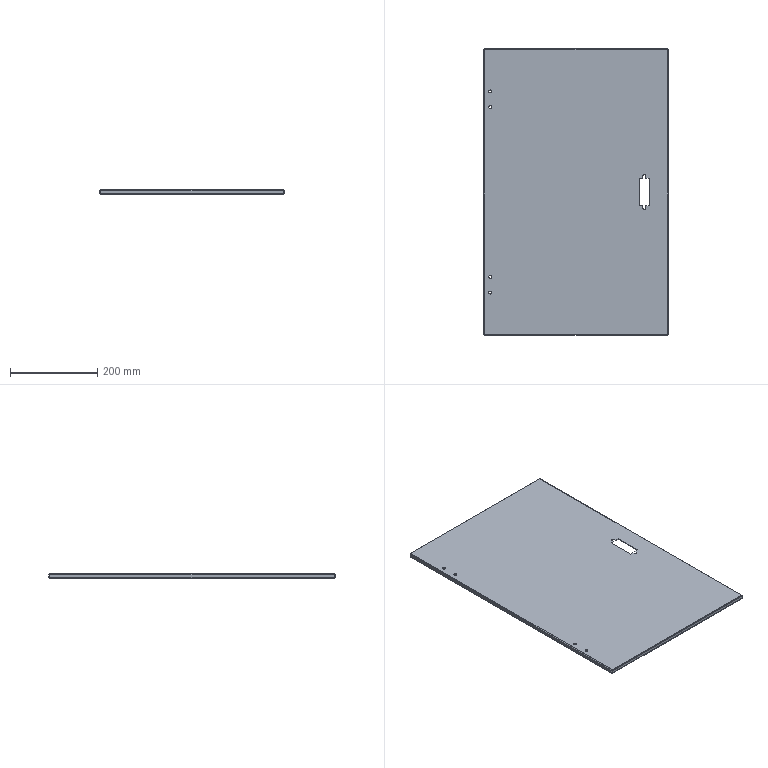Part | SolidWorks | features BaseBody 1 | 1 solid | 90 faces | box 422 x 656 x 10 mm | volume 462657 mm3 | plane 48 | cylinder 26 | spline 16 | commonest cylinder face diameters 1.473 x8 4.473 x8 6.8 x8 6.5 x2